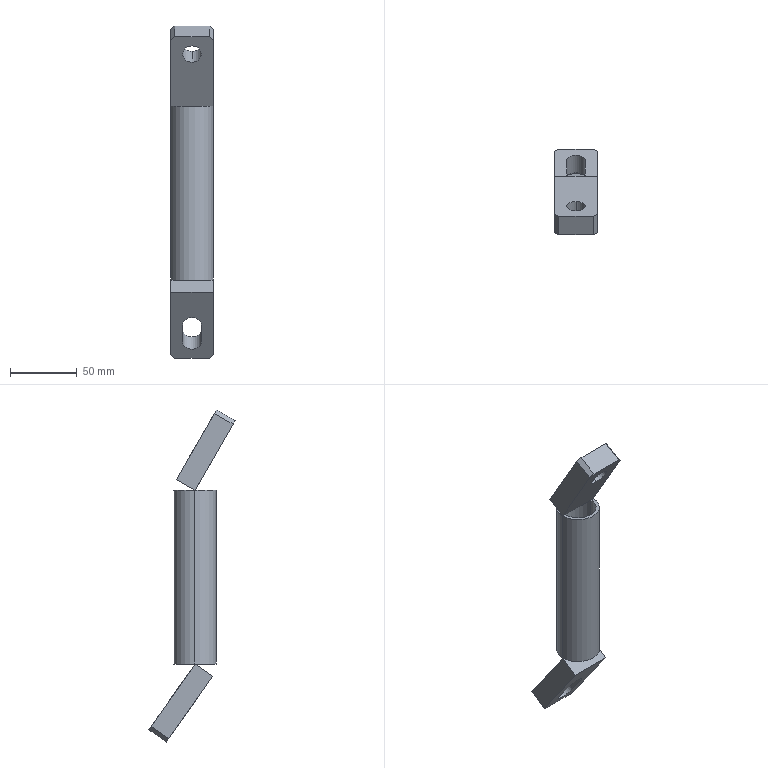Part | SolidWorks | features ICE 4, Chamfer 2, Extrusion 1 | 3 solids | 29 faces | box 32 x 64.415 x 248.288 mm | volume 82986 mm3 | plane 20 | cylinder 9 | commonest cylinder face diameters 14 x5 27 x2 32 x2
STEP:
#1=CARTESIAN_POINT('',(-13.5,0.,130.));
#2=VERTEX_POINT('',#1);
#3=CARTESIAN_POINT('',(13.5,0.,130.));
#4=VERTEX_POINT('',#3);
#5=CARTESIAN_POINT('',(0.,0.,130.));
#6=DIRECTION('',(0.,0.,1.));
#7=DIRECTION('',(1.,0.,0.));
#8=AXIS2_PLACEMENT_3D('',#5,#6,#7);
#9=CIRCLE('',#8,13.5);
#10=EDGE_CURVE('',#2,#4,#9,.T.);
#11=ORIENTED_EDGE('',*,*,#10,.T.);
#12=CARTESIAN_POINT('',(13.5,0.,0.));
#13=VERTEX_POINT('',#12);
#14=CARTESIAN_POINT('',(13.5,0.,130.));
#15=DIRECTION('',(0.,0.,-1.));
#16=VECTOR('',#15,1000.);
#17=LINE('',#14,#16);
#18=EDGE_CURVE('',#4,#13,#17,.T.);
#19=ORIENTED_EDGE('',*,*,#18,.T.);
#20=CARTESIAN_POINT('',(-13.5,0.,0.));
#21=VERTEX_POINT('',#20);
#22=CARTESIAN_POINT('',(0.,0.,0.));
#23=DIRECTION('',(0.,0.,1.));
#24=DIRECTION('',(1.,0.,0.));
#25=AXIS2_PLACEMENT_3D('',#22,#23,#24);
#26=CIRCLE('',#25,13.5);
#27=EDGE_CURVE('',#21,#13,#26,.T.);
#28=ORIENTED_EDGE('',*,*,#27,.F.);
#29=CARTESIAN_POINT('',(-13.5,0.,130.));
#30=DIRECTION('',(0.,0.,-1.));
#31=VECTOR('',#30,1000.);
#32=LINE('',#29,#31);
#33=EDGE_CURVE('',#2,#21,#32,.T.);
#34=ORIENTED_EDGE('',*,*,#33,.F.);
#35=EDGE_LOOP('',(#11,#19,#28,#34));
#36=FACE_OUTER_BOUND('',#35,.T.);
#37=CARTESIAN_POINT('',(0.,0.,130.));
#38=DIRECTION('',(0.,0.,-1.));
#39=DIRECTION('',(-1.,0.,0.));
#40=AXIS2_PLACEMENT_3D('',#37,#38,#39);
#41=CYLINDRICAL_SURFACE('',#40,13.5);
#42=ADVANCED_FACE('',(#36),#41,.F.);
#43=CARTESIAN_POINT('',(16.,0.,130.));
#44=VERTEX_POINT('',#43);
#45=CARTESIAN_POINT('',(-16.,0.,130.));
#46=VERTEX_POINT('',#45);
#47=CARTESIAN_POINT('',(0.,0.,130.));
#48=DIRECTION('',(0.,0.,1.));
#49=DIRECTION('',(1.,0.,0.));
#50=AXIS2_PLACEMENT_3D('',#47,#48,#49);
#51=CIRCLE('',#50,16.);
#52=EDGE_CURVE('',#44,#46,#51,.T.);
#53=ORIENTED_EDGE('',*,*,#52,.F.);
#54=CARTESIAN_POINT('',(16.,0.,0.));
#55=VERTEX_POINT('',#54);
#56=CARTESIAN_POINT('',(16.,0.,130.));
#57=DIRECTION('',(0.,0.,-1.));
#58=VECTOR('',#57,1000.);
#59=LINE('',#56,#58);
#60=EDGE_CURVE('',#44,#55,#59,.T.);
#61=ORIENTED_EDGE('',*,*,#60,.T.);
#62=CARTESIAN_POINT('',(-16.,0.,0.));
#63=VERTEX_POINT('',#62);
#64=CARTESIAN_POINT('',(0.,0.,0.));
#65=DIRECTION('',(0.,0.,1.));
#66=DIRECTION('',(1.,0.,0.));
#67=AXIS2_PLACEMENT_3D('',#64,#65,#66);
#68=CIRCLE('',#67,16.);
#69=EDGE_CURVE('',#55,#63,#68,.T.);
#70=ORIENTED_EDGE('',*,*,#69,.T.);
#71=CARTESIAN_POINT('',(-16.,0.,130.));
#72=DIRECTION('',(0.,0.,-1.));
#73=VECTOR('',#72,1000.);
#74=LINE('',#71,#73);
#75=EDGE_CURVE('',#46,#63,#74,.T.);
#76=ORIENTED_EDGE('',*,*,#75,.F.);
#77=EDGE_LOOP('',(#53,#61,#70,#76));
#78=FACE_OUTER_BOUND('',#77,.T.);
#79=CARTESIAN_POINT('',(0.,0.,130.));
#80=DIRECTION('',(0.,0.,-1.));
#81=DIRECTION('',(-1.,0.,0.));
#82=AXIS2_PLACEMENT_3D('',#79,#80,#81);
#83=CYLINDRICAL_SURFACE('',#82,16.);
#84=ADVANCED_FACE('',(#78),#83,.T.);
#85=CARTESIAN_POINT('',(0.,0.,130.));
#86=DIRECTION('',(0.,0.,1.));
#87=DIRECTION('',(1.,0.,0.));
#88=AXIS2_PLACEMENT_3D('',#85,#86,#87);
#89=CIRCLE('',#88,16.);
#90=EDGE_CURVE('',#46,#44,#89,.T.);
#91=ORIENTED_EDGE('',*,*,#90,.T.);
#92=ORIENTED_EDGE('',*,*,#52,.T.);
#93=EDGE_LOOP('',(#91,#92));
#94=FACE_OUTER_BOUND('',#93,.T.);
#95=ORIENTED_EDGE('',*,*,#10,.F.);
#96=CARTESIAN_POINT('',(0.,0.,130.));
#97=DIRECTION('',(0.,0.,1.));
#98=DIRECTION('',(1.,0.,0.));
#99=AXIS2_PLACEMENT_3D('',#96,#97,#98);
#100=CIRCLE('',#99,13.5);
#101=EDGE_CURVE('',#4,#2,#100,.T.);
#102=ORIENTED_EDGE('',*,*,#101,.F.);
#103=EDGE_LOOP('',(#95,#102));
#104=FACE_BOUND('',#103,.T.);
#105=CARTESIAN_POINT('',(0.,0.,130.));
#106=DIRECTION('',(0.,0.,1.));
#107=DIRECTION('',(1.,0.,0.));
#108=AXIS2_PLACEMENT_3D('',#105,#106,#107);
#109=PLANE('',#108);
#110=ADVANCED_FACE('',(#94,#104),#109,.T.);
#111=CARTESIAN_POINT('',(0.,0.,0.));
#112=DIRECTION('',(0.,0.,1.));
#113=DIRECTION('',(1.,0.,0.));
#114=AXIS2_PLACEMENT_3D('',#111,#112,#113);
#115=CIRCLE('',#114,16.);
#116=EDGE_CURVE('',#63,#55,#115,.T.);
#117=ORIENTED_EDGE('',*,*,#116,.F.);
#118=ORIENTED_EDGE('',*,*,#69,.F.);
#119=EDGE_LOOP('',(#117,#118));
#120=FACE_OUTER_BOUND('',#119,.T.);
#121=ORIENTED_EDGE('',*,*,#27,.T.);
#122=CARTESIAN_POINT('',(0.,0.,0.));
#123=DIRECTION('',(0.,0.,1.));
#124=DIRECTION('',(1.,0.,0.));
#125=AXIS2_PLACEMENT_3D('',#122,#123,#124);
#126=CIRCLE('',#125,13.5);
#127=EDGE_CURVE('',#13,#21,#126,.T.);
#128=ORIENTED_EDGE('',*,*,#127,.T.);
#129=EDGE_LOOP('',(#121,#128));
#130=FACE_BOUND('',#129,.T.);
#131=CARTESIAN_POINT('',(0.,0.,0.));
#132=DIRECTION('',(0.,0.,1.));
#133=DIRECTION('',(1.,0.,0.));
#134=AXIS2_PLACEMENT_3D('',#131,#132,#133);
#135=PLANE('',#134);
#136=ADVANCED_FACE('',(#120,#130),#135,.F.);
#137=ORIENTED_EDGE('',*,*,#60,.F.);
#138=ORIENTED_EDGE('',*,*,#90,.F.);
#139=ORIENTED_EDGE('',*,*,#75,.T.);
#140=ORIENTED_EDGE('',*,*,#116,.T.);
#141=EDGE_LOOP('',(#137,#138,#139,#140));
#142=FACE_OUTER_BOUND('',#141,.T.);
#143=CARTESIAN_POINT('',(0.,0.,130.));
#144=DIRECTION('',(0.,0.,-1.));
#145=DIRECTION('',(-1.,0.,0.));
#146=AXIS2_PLACEMENT_3D('',#143,#144,#145);
#147=CYLINDRICAL_SURFACE('',#146,16.);
#148=ADVANCED_FACE('',(#142),#147,.T.);
#149=ORIENTED_EDGE('',*,*,#18,.F.);
#150=ORIENTED_EDGE('',*,*,#101,.T.);
#151=ORIENTED_EDGE('',*,*,#33,.T.);
#152=ORIENTED_EDGE('',*,*,#127,.F.);
#153=EDGE_LOOP('',(#149,#150,#151,#152));
#154=FACE_OUTER_BOUND('',#153,.T.);
#155=CARTESIAN_POINT('',(0.,0.,130.));
#156=DIRECTION('',(0.,0.,-1.));
#157=DIRECTION('',(-1.,0.,0.));
#158=AXIS2_PLACEMENT_3D('',#155,#156,#157);
#159=CYLINDRICAL_SURFACE('',#158,13.5);
#160=ADVANCED_FACE('',(#154),#159,.F.);
#161=CLOSED_SHELL('',(#42,#84,#110,#136,#148,#160));
#162=MANIFOLD_SOLID_BREP('',#161);
#163=CARTESIAN_POINT('',(0.,0.08583,-28.018));
#164=VERTEX_POINT('',#163);
#165=CARTESIAN_POINT('',(7.,4.101,-33.752));
#166=VERTEX_POINT('',#165);
#167=CARTESIAN_POINT('',(0.,4.101,-33.752));
#168=DIRECTION('',(0.,0.8192,0.5736));
#169=DIRECTION('',(0.,-0.5736,0.8192));
#170=AXIS2_PLACEMENT_3D('',#167,#168,#169);
#171=CIRCLE('',#170,7.);
#172=EDGE_CURVE('',#164,#166,#171,.T.);
#173=ORIENTED_EDGE('',*,*,#172,.F.);
#174=CARTESIAN_POINT('',(0.,13.192,-18.84));
#175=VERTEX_POINT('',#174);
#176=CARTESIAN_POINT('',(0.,-24.948,-45.547));
#177=DIRECTION('',(0.,0.8192,0.5736));
#178=VECTOR('',#177,1000.);
#179=LINE('',#176,#178);
#180=EDGE_CURVE('',#164,#175,#179,.T.);
#181=ORIENTED_EDGE('',*,*,#180,.T.);
#182=CARTESIAN_POINT('',(7.,17.207,-24.575));
#183=VERTEX_POINT('',#182);
#184=CARTESIAN_POINT('',(0.,17.207,-24.575));
#185=DIRECTION('',(0.,0.8192,0.5736));
#186=DIRECTION('',(0.,-0.5736,0.8192));
#187=AXIS2_PLACEMENT_3D('',#184,#185,#186);
#188=CIRCLE('',#187,7.);
#189=EDGE_CURVE('',#175,#183,#188,.T.);
#190=ORIENTED_EDGE('',*,*,#189,.T.);
#191=CARTESIAN_POINT('',(7.,-20.933,-51.281));
#192=DIRECTION('',(0.,0.8192,0.5736));
#193=VECTOR('',#192,1000.);
#194=LINE('',#191,#193);
#195=EDGE_CURVE('',#166,#183,#194,.T.);
#196=ORIENTED_EDGE('',*,*,#195,.F.);
#197=EDGE_LOOP('',(#173,#181,#190,#196));
#198=FACE_OUTER_BOUND('',#197,.T.);
#199=CARTESIAN_POINT('',(0.,-20.933,-51.281));
#200=DIRECTION('',(0.,0.8192,0.5736));
#201=DIRECTION('',(0.,-0.5736,0.8192));
#202=AXIS2_PLACEMENT_3D('',#199,#200,#201);
#203=CYLINDRICAL_SURFACE('',#202,7.);
#204=ADVANCED_FACE('',(#198),#203,.F.);
#205=CARTESIAN_POINT('',(-16.,0.,0.));
#206=VERTEX_POINT('',#205);
#207=CARTESIAN_POINT('',(-16.,-13.106,-9.177));
#208=VERTEX_POINT('',#207);
#209=CARTESIAN_POINT('',(-16.,-13.106,-9.177));
#210=DIRECTION('',(0.,-0.8192,-0.5736));
#211=VECTOR('',#210,1000.);
#212=LINE('',#209,#211);
#213=EDGE_CURVE('',#206,#208,#212,.T.);
#214=ORIENTED_EDGE('',*,*,#213,.T.);
#215=CARTESIAN_POINT('',(16.,-13.106,-9.177));
#216=VERTEX_POINT('',#215);
#217=CARTESIAN_POINT('',(16.,-13.106,-9.177));
#218=DIRECTION('',(-1.,0.,0.));
#219=VECTOR('',#218,1000.);
#220=LINE('',#217,#219);
#221=EDGE_CURVE('',#216,#208,#220,.T.);
#222=ORIENTED_EDGE('',*,*,#221,.F.);
#223=CARTESIAN_POINT('',(16.,0.,0.));
#224=VERTEX_POINT('',#223);
#225=CARTESIAN_POINT('',(16.,-13.106,-9.177));
#226=DIRECTION('',(0.,-0.8192,-0.5736));
#227=VECTOR('',#226,1000.);
#228=LINE('',#225,#227);
#229=EDGE_CURVE('',#224,#216,#228,.T.);
#230=ORIENTED_EDGE('',*,*,#229,.F.);
#231=CARTESIAN_POINT('',(16.,0.,0.));
#232=DIRECTION('',(-1.,0.,0.));
#233=VECTOR('',#232,1000.);
#234=LINE('',#231,#233);
#235=EDGE_CURVE('',#224,#206,#234,.T.);
#236=ORIENTED_EDGE('',*,*,#235,.T.);
#237=EDGE_LOOP('',(#214,#222,#230,#236));
#238=FACE_OUTER_BOUND('',#237,.T.);
#239=CARTESIAN_POINT('',(16.,-13.106,-9.177));
#240=DIRECTION('',(0.,0.5736,-0.8192));
#241=DIRECTION('',(0.,0.8192,0.5736));
#242=AXIS2_PLACEMENT_3D('',#239,#240,#241);
#243=PLANE('',#242);
#244=ADVANCED_FACE('',(#238),#243,.F.);
#245=CARTESIAN_POINT('',(7.,12.705,-46.039));
#246=VERTEX_POINT('',#245);
#247=CARTESIAN_POINT('',(7.,21.308,-58.326));
#248=DIRECTION('',(0.,0.5736,-0.8192));
#249=VECTOR('',#248,1000.);
#250=LINE('',#247,#249);
#251=EDGE_CURVE('',#166,#246,#250,.T.);
#252=ORIENTED_EDGE('',*,*,#251,.T.);
#253=CARTESIAN_POINT('',(-7.,12.705,-46.039));
#254=VERTEX_POINT('',#253);
#255=CARTESIAN_POINT('',(0.,12.705,-46.039));
#256=DIRECTION('',(0.,0.8192,0.5736));
#257=DIRECTION('',(0.,-0.5736,0.8192));
#258=AXIS2_PLACEMENT_3D('',#255,#256,#257);
#259=CIRCLE('',#258,7.);
#260=EDGE_CURVE('',#246,#254,#259,.T.);
#261=ORIENTED_EDGE('',*,*,#260,.T.);
#262=CARTESIAN_POINT('',(-7.,4.101,-33.752));
#263=VERTEX_POINT('',#262);
#264=CARTESIAN_POINT('',(-7.,21.308,-58.326));
#265=DIRECTION('',(0.,-0.5736,0.8192));
#266=VECTOR('',#265,1000.);
#267=LINE('',#264,#266);
#268=EDGE_CURVE('',#254,#263,#267,.T.);
#269=ORIENTED_EDGE('',*,*,#268,.T.);
#270=CARTESIAN_POINT('',(0.,4.101,-33.752));
#271=DIRECTION('',(0.,0.8192,0.5736));
#272=DIRECTION('',(0.,-0.5736,0.8192));
#273=AXIS2_PLACEMENT_3D('',#270,#271,#272);
#274=CIRCLE('',#273,7.);
#275=EDGE_CURVE('',#263,#164,#274,.T.);
#276=ORIENTED_EDGE('',*,*,#275,.T.);
#277=ORIENTED_EDGE('',*,*,#172,.T.);
#278=EDGE_LOOP('',(#252,#261,#269,#276,#277));
#279=FACE_BOUND('',#278,.T.);
#280=CARTESIAN_POINT('',(13.,21.308,-58.326));
#281=VERTEX_POINT('',#280);
#282=CARTESIAN_POINT('',(-13.,21.308,-58.326));
#283=VERTEX_POINT('',#282);
#284=CARTESIAN_POINT('',(16.,21.308,-58.326));
#285=DIRECTION('',(-1.,0.,0.));
#286=VECTOR('',#285,1000.);
#287=LINE('',#284,#286);
#288=EDGE_CURVE('',#281,#283,#287,.T.);
#289=ORIENTED_EDGE('',*,*,#288,.F.);
#290=CARTESIAN_POINT('',(16.,19.587,-55.869));
#291=VERTEX_POINT('',#290);
#292=CARTESIAN_POINT('',(16.,19.587,-55.869));
#293=DIRECTION('',(0.7071,-0.4056,0.5792));
#294=VECTOR('',#293,1000.);
#295=LINE('',#292,#294);
#296=EDGE_CURVE('',#281,#291,#295,.T.);
#297=ORIENTED_EDGE('',*,*,#296,.T.);
#298=CARTESIAN_POINT('',(16.,21.308,-58.326));
#299=DIRECTION('',(0.,0.5736,-0.8192));
#300=VECTOR('',#299,1000.);
#301=LINE('',#298,#300);
#302=EDGE_CURVE('',#216,#291,#301,.T.);
#303=ORIENTED_EDGE('',*,*,#302,.F.);
#304=ORIENTED_EDGE('',*,*,#221,.T.);
#305=CARTESIAN_POINT('',(-16.,19.587,-55.869));
#306=VERTEX_POINT('',#305);
#307=CARTESIAN_POINT('',(-16.,21.308,-58.326));
#308=DIRECTION('',(0.,0.5736,-0.8192));
#309=VECTOR('',#308,1000.);
#310=LINE('',#307,#309);
#311=EDGE_CURVE('',#208,#306,#310,.T.);
#312=ORIENTED_EDGE('',*,*,#311,.T.);
#313=CARTESIAN_POINT('',(-13.,21.308,-58.326));
#314=DIRECTION('',(0.7071,0.4056,-0.5792));
#315=VECTOR('',#314,1000.);
#316=LINE('',#313,#315);
#317=EDGE_CURVE('',#306,#283,#316,.T.);
#318=ORIENTED_EDGE('',*,*,#317,.T.);
#319=EDGE_LOOP('',(#289,#297,#303,#304,#312,#318));
#320=FACE_OUTER_BOUND('',#319,.T.);
#321=CARTESIAN_POINT('',(16.,21.308,-58.326));
#322=DIRECTION('',(0.,0.8192,0.5736));
#323=DIRECTION('',(0.,-0.5736,0.8192));
#324=AXIS2_PLACEMENT_3D('',#321,#322,#323);
#325=PLANE('',#324);
#326=ADVANCED_FACE('',(#279,#320),#325,.F.);
#327=CARTESIAN_POINT('',(13.,34.415,-49.149));
#328=VERTEX_POINT('',#327);
#329=CARTESIAN_POINT('',(-13.,34.415,-49.149));
#330=VERTEX_POINT('',#329);
#331=CARTESIAN_POINT('',(16.,34.415,-49.149));
#332=DIRECTION('',(-1.,0.,0.));
#333=VECTOR('',#332,1000.);
#334=LINE('',#331,#333);
#335=EDGE_CURVE('',#328,#330,#334,.T.);
#336=ORIENTED_EDGE('',*,*,#335,.F.);
#337=CARTESIAN_POINT('',(13.,34.415,-49.149));
#338=DIRECTION('',(0.,-0.8192,-0.5736));
#339=VECTOR('',#338,1000.);
#340=LINE('',#337,#339);
#341=EDGE_CURVE('',#328,#281,#340,.T.);
#342=ORIENTED_EDGE('',*,*,#341,.T.);
#343=ORIENTED_EDGE('',*,*,#288,.T.);
#344=CARTESIAN_POINT('',(-13.,34.415,-49.149));
#345=DIRECTION('',(0.,0.8192,0.5736));
#346=VECTOR('',#345,1000.);
#347=LINE('',#344,#346);
#348=EDGE_CURVE('',#283,#330,#347,.T.);
#349=ORIENTED_EDGE('',*,*,#348,.T.);
#350=EDGE_LOOP('',(#336,#342,#343,#349));
#351=FACE_OUTER_BOUND('',#350,.T.);
#352=CARTESIAN_POINT('',(16.,34.415,-49.149));
#353=DIRECTION('',(0.,-0.5736,0.8192));
#354=DIRECTION('',(0.,-0.8192,-0.5736));
#355=AXIS2_PLACEMENT_3D('',#352,#353,#354);
#356=PLANE('',#355);
#357=ADVANCED_FACE('',(#351),#356,.F.);
#358=CARTESIAN_POINT('',(-7.,25.811,-36.862));
#359=VERTEX_POINT('',#358);
#360=CARTESIAN_POINT('',(-7.,17.207,-24.575));
#361=VERTEX_POINT('',#360);
#362=CARTESIAN_POINT('',(-7.,25.811,-36.862));
#363=DIRECTION('',(0.,-0.5736,0.8192));
#364=VECTOR('',#363,1000.);
#365=LINE('',#362,#364);
#366=EDGE_CURVE('',#359,#361,#365,.T.);
#367=ORIENTED_EDGE('',*,*,#366,.F.);
#368=CARTESIAN_POINT('',(7.,25.811,-36.862));
#369=VERTEX_POINT('',#368);
#370=CARTESIAN_POINT('',(0.,25.811,-36.862));
#371=DIRECTION('',(0.,0.8192,0.5736));
#372=DIRECTION('',(0.,-0.5736,0.8192));
#373=AXIS2_PLACEMENT_3D('',#370,#371,#372);
#374=CIRCLE('',#373,7.);
#375=EDGE_CURVE('',#369,#359,#374,.T.);
#376=ORIENTED_EDGE('',*,*,#375,.F.);
#377=CARTESIAN_POINT('',(7.,25.811,-36.862));
#378=DIRECTION('',(0.,0.5736,-0.8192));
#379=VECTOR('',#378,1000.);
#380=LINE('',#377,#379);
#381=EDGE_CURVE('',#183,#369,#380,.T.);
#382=ORIENTED_EDGE('',*,*,#381,.F.);
#383=ORIENTED_EDGE('',*,*,#189,.F.);
#384=CARTESIAN_POINT('',(0.,17.207,-24.575));
#385=DIRECTION('',(0.,0.8192,0.5736));
#386=DIRECTION('',(0.,-0.5736,0.8192));
#387=AXIS2_PLACEMENT_3D('',#384,#385,#386);
#388=CIRCLE('',#387,7.);
#389=EDGE_CURVE('',#361,#175,#388,.T.);
#390=ORIENTED_EDGE('',*,*,#389,.F.);
#391=EDGE_LOOP('',(#367,#376,#382,#383,#390));
#392=FACE_BOUND('',#391,.T.);
#393=CARTESIAN_POINT('',(16.,32.694,-46.692));
#394=VERTEX_POINT('',#393);
#395=CARTESIAN_POINT('',(16.,0.,0.));
#396=DIRECTION('',(0.,-0.5736,0.8192));
#397=VECTOR('',#396,1000.);
#398=LINE('',#395,#397);
#399=EDGE_CURVE('',#394,#224,#398,.T.);
#400=ORIENTED_EDGE('',*,*,#399,.F.);
#401=CARTESIAN_POINT('',(16.,32.694,-46.692));
#402=DIRECTION('',(-0.7071,0.4056,-0.5792));
#403=VECTOR('',#402,1000.);
#404=LINE('',#401,#403);
#405=EDGE_CURVE('',#394,#328,#404,.T.);
#406=ORIENTED_EDGE('',*,*,#405,.T.);
#407=ORIENTED_EDGE('',*,*,#335,.T.);
#408=CARTESIAN_POINT('',(-16.,32.694,-46.692));
#409=VERTEX_POINT('',#408);
#410=CARTESIAN_POINT('',(-13.,34.415,-49.149));
#411=DIRECTION('',(-0.7071,-0.4056,0.5792));
#412=VECTOR('',#411,1000.);
#413=LINE('',#410,#412);
#414=EDGE_CURVE('',#330,#409,#413,.T.);
#415=ORIENTED_EDGE('',*,*,#414,.T.);
#416=CARTESIAN_POINT('',(-16.,0.,0.));
#417=DIRECTION('',(0.,-0.5736,0.8192));
#418=VECTOR('',#417,1000.);
#419=LINE('',#416,#418);
#420=EDGE_CURVE('',#409,#206,#419,.T.);
#421=ORIENTED_EDGE('',*,*,#420,.T.);
#422=ORIENTED_EDGE('',*,*,#235,.F.);
#423=EDGE_LOOP('',(#400,#406,#407,#415,#421,#422));
#424=FACE_OUTER_BOUND('',#423,.T.);
#425=CARTESIAN_POINT('',(16.,0.,0.));
#426=DIRECTION('',(0.,-0.8192,-0.5736));
#427=DIRECTION('',(0.,0.5736,-0.8192));
#428=AXIS2_PLACEMENT_3D('',#425,#426,#427);
#429=PLANE('',#428);
#430=ADVANCED_FACE('',(#392,#424),#429,.F.);
#431=ORIENTED_EDGE('',*,*,#302,.T.);
#432=CARTESIAN_POINT('',(16.,32.694,-46.692));
#433=DIRECTION('',(0.,0.8192,0.5736));
#434=VECTOR('',#433,1000.);
#435=LINE('',#432,#434);
#436=EDGE_CURVE('',#291,#394,#435,.T.);
#437=ORIENTED_EDGE('',*,*,#436,.T.);
#438=ORIENTED_EDGE('',*,*,#399,.T.);
#439=ORIENTED_EDGE('',*,*,#229,.T.);
#440=EDGE_LOOP('',(#431,#437,#438,#439));
#441=FACE_OUTER_BOUND('',#440,.T.);
#442=CARTESIAN_POINT('',(16.,0.,0.));
#443=DIRECTION('',(-1.,0.,0.));
#444=DIRECTION('',(0.,0.,1.));
#445=AXIS2_PLACEMENT_3D('',#442,#443,#444);
#446=PLANE('',#445);
#447=ADVANCED_FACE('',(#441),#446,.F.);
#448=ORIENTED_EDGE('',*,*,#420,.F.);
#449=CARTESIAN_POINT('',(-16.,19.587,-55.869));
#450=DIRECTION('',(0.,-0.8192,-0.5736));
#451=VECTOR('',#450,1000.);
#452=LINE('',#449,#451);
#453=EDGE_CURVE('',#409,#306,#452,.T.);
#454=ORIENTED_EDGE('',*,*,#453,.T.);
#455=ORIENTED_EDGE('',*,*,#311,.F.);
#456=ORIENTED_EDGE('',*,*,#213,.F.);
#457=EDGE_LOOP('',(#448,#454,#455,#456));
#458=FACE_OUTER_BOUND('',#457,.T.);
#459=CARTESIAN_POINT('',(-16.,0.,0.));
#460=DIRECTION('',(-1.,0.,0.));
#461=DIRECTION('',(0.,0.,1.));
#462=AXIS2_PLACEMENT_3D('',#459,#460,#461);
#463=PLANE('',#462);
#464=ADVANCED_FACE('',(#458),#463,.T.);
#465=CARTESIAN_POINT('',(7.,-12.33,-63.568));
#466=DIRECTION('',(0.,0.8192,0.5736));
#467=VECTOR('',#466,1000.);
#468=LINE('',#465,#467);
#469=EDGE_CURVE('',#246,#369,#468,.T.);
#470=ORIENTED_EDGE('',*,*,#469,.T.);
#471=ORIENTED_EDGE('',*,*,#375,.T.);
#472=CARTESIAN_POINT('',(-7.,-12.33,-63.568));
#473=DIRECTION('',(0.,0.8192,0.5736));
#474=VECTOR('',#473,1000.);
#475=LINE('',#472,#474);
#476=EDGE_CURVE('',#254,#359,#475,.T.);
#477=ORIENTED_EDGE('',*,*,#476,.F.);
#478=ORIENTED_EDGE('',*,*,#260,.F.);
#479=EDGE_LOOP('',(#470,#471,#477,#478));
#480=FACE_OUTER_BOUND('',#479,.T.);
#481=CARTESIAN_POINT('',(0.,-12.33,-63.568));
#482=DIRECTION('',(0.,0.8192,0.5736));
#483=DIRECTION('',(0.,-0.5736,0.8192));
#484=AXIS2_PLACEMENT_3D('',#481,#482,#483);
#485=CYLINDRICAL_SURFACE('',#484,7.);
#486=ADVANCED_FACE('',(#480),#485,.F.);
#487=ORIENTED_EDGE('',*,*,#195,.T.);
#488=ORIENTED_EDGE('',*,*,#381,.T.);
#489=ORIENTED_EDGE('',*,*,#469,.F.);
#490=ORIENTED_EDGE('',*,*,#251,.F.);
#491=EDGE_LOOP('',(#487,#488,#489,#490));
#492=FACE_OUTER_BOUND('',#491,.T.);
#493=CARTESIAN_POINT('',(7.,-12.33,-63.568));
#494=DIRECTION('',(1.,0.,0.));
#495=DIRECTION('',(0.,0.,-1.));
#496=AXIS2_PLACEMENT_3D('',#493,#494,#495);
#497=PLANE('',#496);
#498=ADVANCED_FACE('',(#492),#497,.F.);
#499=ORIENTED_EDGE('',*,*,#180,.F.);
#500=ORIENTED_EDGE('',*,*,#275,.F.);
#501=CARTESIAN_POINT('',(-7.,-20.933,-51.281));
#502=DIRECTION('',(0.,0.8192,0.5736));
#503=VECTOR('',#502,1000.);
#504=LINE('',#501,#503);
#505=EDGE_CURVE('',#263,#361,#504,.T.);
#506=ORIENTED_EDGE('',*,*,#505,.T.);
#507=ORIENTED_EDGE('',*,*,#389,.T.);
#508=EDGE_LOOP('',(#499,#500,#506,#507));
#509=FACE_OUTER_BOUND('',#508,.T.);
#510=CARTESIAN_POINT('',(0.,-20.933,-51.281));
#511=DIRECTION('',(0.,0.8192,0.5736));
#512=DIRECTION('',(0.,-0.5736,0.8192));
#513=AXIS2_PLACEMENT_3D('',#510,#511,#512);
#514=CYLINDRICAL_SURFACE('',#513,7.);
#515=ADVANCED_FACE('',(#509),#514,.F.);
#516=ORIENTED_EDGE('',*,*,#476,.T.);
#517=ORIENTED_EDGE('',*,*,#366,.T.);
#518=ORIENTED_EDGE('',*,*,#505,.F.);
#519=ORIENTED_EDGE('',*,*,#268,.F.);
#520=EDGE_LOOP('',(#516,#517,#518,#519));
#521=FACE_OUTER_BOUND('',#520,.T.);
#522=CARTESIAN_POINT('',(-7.,-12.33,-63.568));
#523=DIRECTION('',(-1.,0.,0.));
#524=DIRECTION('',(0.,0.,1.));
#525=AXIS2_PLACEMENT_3D('',#522,#523,#524);
#526=PLANE('',#525);
#527=ADVANCED_FACE('',(#521),#526,.F.);
#528=ORIENTED_EDGE('',*,*,#296,.F.);
#529=ORIENTED_EDGE('',*,*,#341,.F.);
#530=ORIENTED_EDGE('',*,*,#405,.F.);
#531=ORIENTED_EDGE('',*,*,#436,.F.);
#532=EDGE_LOOP('',(#528,#529,#530,#531));
#533=FACE_OUTER_BOUND('',#532,.T.);
#534=CARTESIAN_POINT('',(16.,32.694,-46.692));
#535=DIRECTION('',(-0.7071,-0.4056,0.5792));
#536=DIRECTION('',(0.,0.8192,0.5736));
#537=AXIS2_PLACEMENT_3D('',#534,#535,#536);
#538=PLANE('',#537);
#539=ADVANCED_FACE('',(#533),#538,.F.);
#540=ORIENTED_EDGE('',*,*,#317,.F.);
#541=ORIENTED_EDGE('',*,*,#453,.F.);
#542=ORIENTED_EDGE('',*,*,#414,.F.);
#543=ORIENTED_EDGE('',*,*,#348,.F.);
#544=EDGE_LOOP('',(#540,#541,#542,#543));
#545=FACE_OUTER_BOUND('',#544,.T.);
#546=CARTESIAN_POINT('',(-13.,34.415,-49.149));
#547=DIRECTION('',(-0.7071,0.4056,-0.5792));
#548=DIRECTION('',(0.,-0.8192,-0.5736));
#549=AXIS2_PLACEMENT_3D('',#546,#547,#548);
#550=PLANE('',#549);
#551=ADVANCED_FACE('',(#545),#550,.T.);
#552=CLOSED_SHELL('',(#204,#244,#326,#357,#430,#447,#464,#486,#498,#515,#527,#539,#551));
#553=MANIFOLD_SOLID_BREP('',#552);
#554=CARTESIAN_POINT('',(0.,-12.144,183.033));
#555=VERTEX_POINT('',#554);
#556=CARTESIAN_POINT('',(0.,-5.144,170.909));
#557=VERTEX_POINT('',#556);
#558=CARTESIAN_POINT('',(0.,-8.644,176.971));
#559=DIRECTION('',(0.,-0.866,-0.5));
#560=DIRECTION('',(0.,0.5,-0.866));
#561=AXIS2_PLACEMENT_3D('',#558,#559,#560);
#562=CIRCLE('',#561,7.);
#563=EDGE_CURVE('',#555,#557,#562,.T.);
#564=ORIENTED_EDGE('',*,*,#563,.F.);
#565=CARTESIAN_POINT('',(0.,-26.,175.033));
#566=VERTEX_POINT('',#565);
#567=CARTESIAN_POINT('',(0.,25.775,204.926));
#568=DIRECTION('',(0.,-0.866,-0.5));
#569=VECTOR('',#568,1000.);
#570=LINE('',#567,#569);
#571=EDGE_CURVE('',#555,#566,#570,.T.);
#572=ORIENTED_EDGE('',*,*,#571,.T.);
#573=CARTESIAN_POINT('',(0.,-19.,162.909));
#574=VERTEX_POINT('',#573);
#575=CARTESIAN_POINT('',(0.,-22.5,168.971));
#576=DIRECTION('',(0.,-0.866,-0.5));
#577=DIRECTION('',(0.,0.5,-0.866));
#578=AXIS2_PLACEMENT_3D('',#575,#576,#577);
#579=CIRCLE('',#578,7.);
#580=EDGE_CURVE('',#566,#574,#579,.T.);
#581=ORIENTED_EDGE('',*,*,#580,.T.);
#582=CARTESIAN_POINT('',(0.,32.775,192.801));
#583=DIRECTION('',(0.,-0.866,-0.5));
#584=VECTOR('',#583,1000.);
#585=LINE('',#582,#584);
#586=EDGE_CURVE('',#557,#574,#585,.T.);
#587=ORIENTED_EDGE('',*,*,#586,.F.);
#588=EDGE_LOOP('',(#564,#572,#581,#587));
#589=FACE_OUTER_BOUND('',#588,.T.);
#590=CARTESIAN_POINT('',(0.,29.275,198.863));
#591=DIRECTION('',(0.,-0.866,-0.5));
#592=DIRECTION('',(0.,0.5,-0.866));
#593=AXIS2_PLACEMENT_3D('',#590,#591,#592);
#594=CYLINDRICAL_SURFACE('',#593,7.);
#595=ADVANCED_FACE('',(#589),#594,.F.);
#596=CARTESIAN_POINT('',(-16.,0.,130.));
#597=VERTEX_POINT('',#596);
#598=CARTESIAN_POINT('',(-16.,13.856,138.));
#599=VERTEX_POINT('',#598);
#600=CARTESIAN_POINT('',(-16.,13.856,138.));
#601=DIRECTION('',(0.,0.866,0.5));
#602=VECTOR('',#601,1000.);
#603=LINE('',#600,#602);
#604=EDGE_CURVE('',#597,#599,#603,.T.);
#605=ORIENTED_EDGE('',*,*,#604,.T.);
#606=CARTESIAN_POINT('',(16.,13.856,138.));
#607=VERTEX_POINT('',#606);
#608=CARTESIAN_POINT('',(16.,13.856,138.));
#609=DIRECTION('',(-1.,0.,0.));
#610=VECTOR('',#609,1000.);
#611=LINE('',#608,#610);
#612=EDGE_CURVE('',#607,#599,#611,.T.);
#613=ORIENTED_EDGE('',*,*,#612,.F.);
#614=CARTESIAN_POINT('',(16.,0.,130.));
#615=VERTEX_POINT('',#614);
#616=CARTESIAN_POINT('',(16.,13.856,138.));
#617=DIRECTION('',(0.,0.866,0.5));
#618=VECTOR('',#617,1000.);
#619=LINE('',#616,#618);
#620=EDGE_CURVE('',#615,#607,#619,.T.);
#621=ORIENTED_EDGE('',*,*,#620,.F.);
#622=CARTESIAN_POINT('',(16.,0.,130.));
#623=DIRECTION('',(-1.,0.,0.));
#624=VECTOR('',#623,1000.);
#625=LINE('',#622,#624);
#626=EDGE_CURVE('',#615,#597,#625,.T.);
#627=ORIENTED_EDGE('',*,*,#626,.T.);
#628=EDGE_LOOP('',(#605,#613,#621,#627));
#629=FACE_OUTER_BOUND('',#628,.T.);
#630=CARTESIAN_POINT('',(16.,13.856,138.));
#631=DIRECTION('',(0.,-0.5,0.866));
#632=DIRECTION('',(0.,-0.866,-0.5));
#633=AXIS2_PLACEMENT_3D('',#630,#631,#632);
#634=PLANE('',#633);
#635=ADVANCED_FACE('',(#629),#634,.F.);
#636=CARTESIAN_POINT('',(0.,-8.644,176.971));
#637=DIRECTION('',(0.,-0.866,-0.5));
#638=DIRECTION('',(0.,0.5,-0.866));
#639=AXIS2_PLACEMENT_3D('',#636,#637,#638);
#640=CIRCLE('',#639,7.);
#641=EDGE_CURVE('',#557,#555,#640,.T.);
#642=ORIENTED_EDGE('',*,*,#641,.T.);
#643=ORIENTED_EDGE('',*,*,#563,.T.);
#644=EDGE_LOOP('',(#642,#643));
#645=FACE_BOUND('',#644,.T.);
#646=CARTESIAN_POINT('',(13.,-16.144,189.962));
#647=VERTEX_POINT('',#646);
#648=CARTESIAN_POINT('',(-13.,-16.144,189.962));
#649=VERTEX_POINT('',#648);
#650=CARTESIAN_POINT('',(16.,-16.144,189.962));
#651=DIRECTION('',(-1.,0.,0.));
#652=VECTOR('',#651,1000.);
#653=LINE('',#650,#652);
#654=EDGE_CURVE('',#647,#649,#653,.T.);
#655=ORIENTED_EDGE('',*,*,#654,.F.);
#656=CARTESIAN_POINT('',(16.,-14.644,187.363));
#657=VERTEX_POINT('',#656);
#658=CARTESIAN_POINT('',(16.,-14.644,187.363));
#659=DIRECTION('',(0.7071,0.3536,-0.6124));
#660=VECTOR('',#659,1000.);
#661=LINE('',#658,#660);
#662=EDGE_CURVE('',#647,#657,#661,.T.);
#663=ORIENTED_EDGE('',*,*,#662,.T.);
#664=CARTESIAN_POINT('',(16.,-16.144,189.962));
#665=DIRECTION('',(0.,-0.5,0.866));
#666=VECTOR('',#665,1000.);
#667=LINE('',#664,#666);
#668=EDGE_CURVE('',#607,#657,#667,.T.);
#669=ORIENTED_EDGE('',*,*,#668,.F.);
#670=ORIENTED_EDGE('',*,*,#612,.T.);
#671=CARTESIAN_POINT('',(-16.,-14.644,187.363));
#672=VERTEX_POINT('',#671);
#673=CARTESIAN_POINT('',(-16.,-16.144,189.962));
#674=DIRECTION('',(0.,-0.5,0.866));
#675=VECTOR('',#674,1000.);
#676=LINE('',#673,#675);
#677=EDGE_CURVE('',#599,#672,#676,.T.);
#678=ORIENTED_EDGE('',*,*,#677,.T.);
#679=CARTESIAN_POINT('',(-13.,-16.144,189.962));
#680=DIRECTION('',(0.7071,-0.3536,0.6124));
#681=VECTOR('',#680,1000.);
#682=LINE('',#679,#681);
#683=EDGE_CURVE('',#672,#649,#682,.T.);
#684=ORIENTED_EDGE('',*,*,#683,.T.);
#685=EDGE_LOOP('',(#655,#663,#669,#670,#678,#684));
#686=FACE_OUTER_BOUND('',#685,.T.);
#687=CARTESIAN_POINT('',(16.,-16.144,189.962));
#688=DIRECTION('',(0.,-0.866,-0.5));
#689=DIRECTION('',(0.,0.5,-0.866));
#690=AXIS2_PLACEMENT_3D('',#687,#688,#689);
#691=PLANE('',#690);
#692=ADVANCED_FACE('',(#645,#686),#691,.F.);
#693=CARTESIAN_POINT('',(13.,-30.,181.962));
#694=VERTEX_POINT('',#693);
#695=CARTESIAN_POINT('',(-13.,-30.,181.962));
#696=VERTEX_POINT('',#695);
#697=CARTESIAN_POINT('',(16.,-30.,181.962));
#698=DIRECTION('',(-1.,0.,0.));
#699=VECTOR('',#698,1000.);
#700=LINE('',#697,#699);
#701=EDGE_CURVE('',#694,#696,#700,.T.);
#702=ORIENTED_EDGE('',*,*,#701,.F.);
#703=CARTESIAN_POINT('',(13.,-16.144,189.962));
#704=DIRECTION('',(0.,0.866,0.5));
#705=VECTOR('',#704,1000.);
#706=LINE('',#703,#705);
#707=EDGE_CURVE('',#694,#647,#706,.T.);
#708=ORIENTED_EDGE('',*,*,#707,.T.);
#709=ORIENTED_EDGE('',*,*,#654,.T.);
#710=CARTESIAN_POINT('',(-13.,-16.144,189.962));
#711=DIRECTION('',(0.,-0.866,-0.5));
#712=VECTOR('',#711,1000.);
#713=LINE('',#710,#712);
#714=EDGE_CURVE('',#649,#696,#713,.T.);
#715=ORIENTED_EDGE('',*,*,#714,.T.);
#716=EDGE_LOOP('',(#702,#708,#709,#715));
#717=FACE_OUTER_BOUND('',#716,.T.);
#718=CARTESIAN_POINT('',(16.,-16.144,189.962));
#719=DIRECTION('',(0.,0.5,-0.866));
#720=DIRECTION('',(0.,0.866,0.5));
#721=AXIS2_PLACEMENT_3D('',#718,#719,#720);
#722=PLANE('',#721);
#723=ADVANCED_FACE('',(#717),#722,.F.);
#724=CARTESIAN_POINT('',(0.,-22.5,168.971));
#725=DIRECTION('',(0.,-0.866,-0.5));
#726=DIRECTION('',(0.,0.5,-0.866));
#727=AXIS2_PLACEMENT_3D('',#724,#725,#726);
#728=CIRCLE('',#727,7.);
#729=EDGE_CURVE('',#574,#566,#728,.T.);
#730=ORIENTED_EDGE('',*,*,#729,.F.);
#731=ORIENTED_EDGE('',*,*,#580,.F.);
#732=EDGE_LOOP('',(#730,#731));
#733=FACE_BOUND('',#732,.T.);
#734=CARTESIAN_POINT('',(16.,-28.5,179.363));
#735=VERTEX_POINT('',#734);
#736=CARTESIAN_POINT('',(16.,-30.,181.962));
#737=DIRECTION('',(0.,0.5,-0.866));
#738=VECTOR('',#737,1000.);
#739=LINE('',#736,#738);
#740=EDGE_CURVE('',#735,#615,#739,.T.);
#741=ORIENTED_EDGE('',*,*,#740,.F.);
#742=CARTESIAN_POINT('',(16.,-28.5,179.363));
#743=DIRECTION('',(-0.7071,-0.3536,0.6124));
#744=VECTOR('',#743,1000.);
#745=LINE('',#742,#744);
#746=EDGE_CURVE('',#735,#694,#745,.T.);
#747=ORIENTED_EDGE('',*,*,#746,.T.);
#748=ORIENTED_EDGE('',*,*,#701,.T.);
#749=CARTESIAN_POINT('',(-16.,-28.5,179.363));
#750=VERTEX_POINT('',#749);
#751=CARTESIAN_POINT('',(-13.,-30.,181.962));
#752=DIRECTION('',(-0.7071,0.3536,-0.6124));
#753=VECTOR('',#752,1000.);
#754=LINE('',#751,#753);
#755=EDGE_CURVE('',#696,#750,#754,.T.);
#756=ORIENTED_EDGE('',*,*,#755,.T.);
#757=CARTESIAN_POINT('',(-16.,-30.,181.962));
#758=DIRECTION('',(0.,0.5,-0.866));
#759=VECTOR('',#758,1000.);
#760=LINE('',#757,#759);
#761=EDGE_CURVE('',#750,#597,#760,.T.);
#762=ORIENTED_EDGE('',*,*,#761,.T.);
#763=ORIENTED_EDGE('',*,*,#626,.F.);
#764=EDGE_LOOP('',(#741,#747,#748,#756,#762,#763));
#765=FACE_OUTER_BOUND('',#764,.T.);
#766=CARTESIAN_POINT('',(16.,-30.,181.962));
#767=DIRECTION('',(0.,0.866,0.5));
#768=DIRECTION('',(0.,-0.5,0.866));
#769=AXIS2_PLACEMENT_3D('',#766,#767,#768);
#770=PLANE('',#769);
#771=ADVANCED_FACE('',(#733,#765),#770,.F.);
#772=ORIENTED_EDGE('',*,*,#668,.T.);
#773=CARTESIAN_POINT('',(16.,-28.5,179.363));
#774=DIRECTION('',(0.,-0.866,-0.5));
#775=VECTOR('',#774,1000.);
#776=LINE('',#773,#775);
#777=EDGE_CURVE('',#657,#735,#776,.T.);
#778=ORIENTED_EDGE('',*,*,#777,.T.);
#779=ORIENTED_EDGE('',*,*,#740,.T.);
#780=ORIENTED_EDGE('',*,*,#620,.T.);
#781=EDGE_LOOP('',(#772,#778,#779,#780));
#782=FACE_OUTER_BOUND('',#781,.T.);
#783=CARTESIAN_POINT('',(16.,0.,0.));
#784=DIRECTION('',(1.,0.,0.));
#785=DIRECTION('',(0.,0.,-1.));
#786=AXIS2_PLACEMENT_3D('',#783,#784,#785);
#787=PLANE('',#786);
#788=ADVANCED_FACE('',(#782),#787,.T.);
#789=ORIENTED_EDGE('',*,*,#761,.F.);
#790=CARTESIAN_POINT('',(-16.,-84.792,146.863));
#791=DIRECTION('',(0.,0.866,0.5));
#792=VECTOR('',#791,1000.);
#793=LINE('',#790,#792);
#794=EDGE_CURVE('',#750,#672,#793,.T.);
#795=ORIENTED_EDGE('',*,*,#794,.T.);
#796=ORIENTED_EDGE('',*,*,#677,.F.);
#797=ORIENTED_EDGE('',*,*,#604,.F.);
#798=EDGE_LOOP('',(#789,#795,#796,#797));
#799=FACE_OUTER_BOUND('',#798,.T.);
#800=CARTESIAN_POINT('',(-16.,0.,0.));
#801=DIRECTION('',(1.,0.,0.));
#802=DIRECTION('',(0.,0.,-1.));
#803=AXIS2_PLACEMENT_3D('',#800,#801,#802);
#804=PLANE('',#803);
#805=ADVANCED_FACE('',(#799),#804,.F.);
#806=ORIENTED_EDGE('',*,*,#571,.F.);
#807=ORIENTED_EDGE('',*,*,#641,.F.);
#808=ORIENTED_EDGE('',*,*,#586,.T.);
#809=ORIENTED_EDGE('',*,*,#729,.T.);
#810=EDGE_LOOP('',(#806,#807,#808,#809));
#811=FACE_OUTER_BOUND('',#810,.T.);
#812=CARTESIAN_POINT('',(0.,29.275,198.863));
#813=DIRECTION('',(0.,-0.866,-0.5));
#814=DIRECTION('',(0.,0.5,-0.866));
#815=AXIS2_PLACEMENT_3D('',#812,#813,#814);
#816=CYLINDRICAL_SURFACE('',#815,7.);
#817=ADVANCED_FACE('',(#811),#816,.F.);
#818=ORIENTED_EDGE('',*,*,#662,.F.);
#819=ORIENTED_EDGE('',*,*,#707,.F.);
#820=ORIENTED_EDGE('',*,*,#746,.F.);
#821=ORIENTED_EDGE('',*,*,#777,.F.);
#822=EDGE_LOOP('',(#818,#819,#820,#821));
#823=FACE_OUTER_BOUND('',#822,.T.);
#824=CARTESIAN_POINT('',(16.,-84.792,146.863));
#825=DIRECTION('',(0.7071,-0.3536,0.6124));
#826=DIRECTION('',(0.,0.866,0.5));
#827=AXIS2_PLACEMENT_3D('',#824,#825,#826);
#828=PLANE('',#827);
#829=ADVANCED_FACE('',(#823),#828,.T.);
#830=ORIENTED_EDGE('',*,*,#683,.F.);
#831=ORIENTED_EDGE('',*,*,#794,.F.);
#832=ORIENTED_EDGE('',*,*,#755,.F.);
#833=ORIENTED_EDGE('',*,*,#714,.F.);
#834=EDGE_LOOP('',(#830,#831,#832,#833));
#835=FACE_OUTER_BOUND('',#834,.T.);
#836=CARTESIAN_POINT('',(-13.,-16.144,189.962));
#837=DIRECTION('',(0.7071,0.3536,-0.6124));
#838=DIRECTION('',(0.,-0.866,-0.5));
#839=AXIS2_PLACEMENT_3D('',#836,#837,#838);
#840=PLANE('',#839);
#841=ADVANCED_FACE('',(#835),#840,.F.);
#842=CLOSED_SHELL('',(#595,#635,#692,#723,#771,#788,#805,#817,#829,#841));
#843=MANIFOLD_SOLID_BREP('',#842);
#844=CARTESIAN_POINT('',(0.,0.,0.));
#845=DIRECTION('',(0.,0.,1.));
#846=DIRECTION('',(1.,0.,0.));
#847=AXIS2_PLACEMENT_3D('',#844,#845,#846);
#848=(LENGTH_UNIT()NAMED_UNIT(*)SI_UNIT(.MILLI.,.METRE.));
#849=UNCERTAINTY_MEASURE_WITH_UNIT(LENGTH_MEASURE(0.00001),#848,'','');
#850=(NAMED_UNIT(*)PLANE_ANGLE_UNIT()SI_UNIT($,.RADIAN.));
#851=(NAMED_UNIT(*)SI_UNIT($,.STERADIAN.)SOLID_ANGLE_UNIT());
#852=(GEOMETRIC_REPRESENTATION_CONTEXT(3)GLOBAL_UNCERTAINTY_ASSIGNED_CONTEXT((#849))GLOBAL_UNIT_ASSIGNED_CONTEXT((#848,#850,#851))REPRESENTATION_CONTEXT('',''));
#853=ADVANCED_BREP_SHAPE_REPRESENTATION('',(#162,#553,#843,#847),#852);